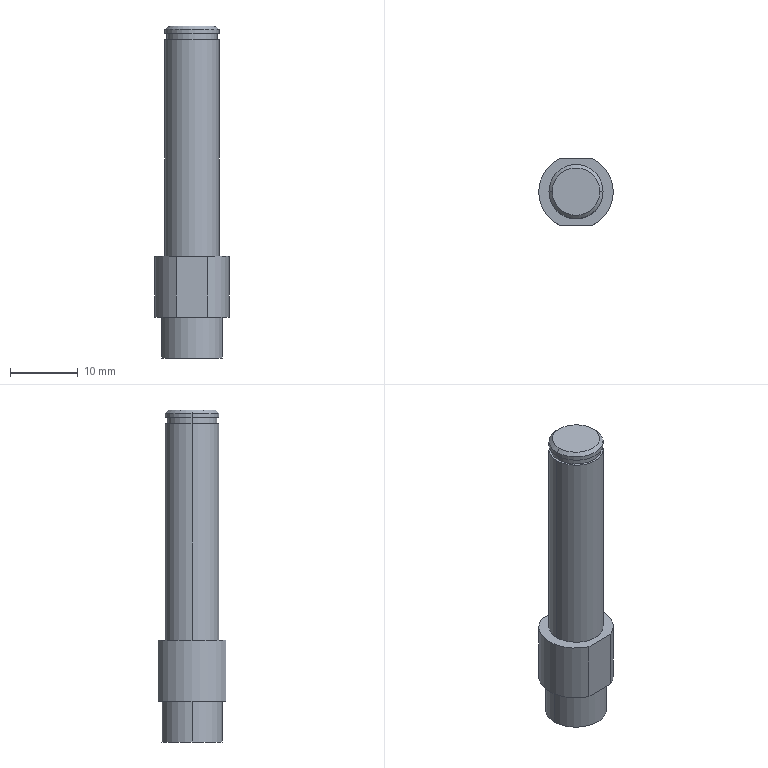Part | STEP file | QA-FC02 | 1 solid | 25 faces | box 11 x 10 x 49 mm | volume 2709 mm3 | cylinder 13 | plane 8 | cone 4 | commonest cylinder face diameters 8 x4 11 x3 4.2 x2 7.4 x2 9 x2
STEP:
#1=CARTESIAN_POINT('',(0.,0.,0.));
#2=DIRECTION('',(0.,0.,1.));
#3=DIRECTION('',(1.,0.,0.));
#4=AXIS2_PLACEMENT_3D('',#1,#2,#3);
#5=CARTESIAN_POINT('',(3.5,0.,34.));
#6=VERTEX_POINT('',#5);
#7=CARTESIAN_POINT('',(-3.5,0.,34.));
#8=VERTEX_POINT('',#7);
#9=CARTESIAN_POINT('',(0.,0.,34.));
#10=DIRECTION('',(0.,0.,1.));
#11=DIRECTION('',(1.,0.,0.));
#12=AXIS2_PLACEMENT_3D('',#9,#10,#11);
#13=CIRCLE('',#12,3.5);
#14=CARTESIAN_POINT('',(0.,0.,34.));
#15=DIRECTION('',(0.,0.,-1.));
#16=DIRECTION('',(-1.,0.,0.));
#17=AXIS2_PLACEMENT_3D('',#14,#15,#16);
#18=CONICAL_SURFACE('',#17,3.5,0.7854);
#19=CARTESIAN_POINT('',(3.142,0.));
#20=DIRECTION('',(-1.,0.));
#21=VECTOR('',#20,1.);
#22=LINE('',#19,#21);
#23=(GEOMETRIC_REPRESENTATION_CONTEXT(2)PARAMETRIC_REPRESENTATION_CONTEXT()REPRESENTATION_CONTEXT('',''));
#24=DEFINITIONAL_REPRESENTATION('',(#22),#23);
#25=PCURVE('',#18,#24);
#26=CARTESIAN_POINT('',(0.,0.,34.));
#27=DIRECTION('',(0.,0.,1.));
#28=DIRECTION('',(1.,0.,0.));
#29=AXIS2_PLACEMENT_3D('',#26,#27,#28);
#30=PLANE('',#29);
#31=CARTESIAN_POINT('',(0.,0.));
#32=DIRECTION('',(1.,0.));
#33=AXIS2_PLACEMENT_2D('',#31,#32);
#34=CIRCLE('',#33,3.5);
#35=(GEOMETRIC_REPRESENTATION_CONTEXT(2)PARAMETRIC_REPRESENTATION_CONTEXT()REPRESENTATION_CONTEXT('',''));
#36=DEFINITIONAL_REPRESENTATION('',(#34),#35);
#37=PCURVE('',#30,#36);
#38=SURFACE_CURVE('',#13,(#25,#37),.PCURVE_S1.);
#39=EDGE_CURVE('',#6,#8,#38,.T.);
#40=ORIENTED_EDGE('',*,*,#39,.F.);
#41=CARTESIAN_POINT('',(4.,0.,33.5));
#42=VERTEX_POINT('',#41);
#43=CARTESIAN_POINT('',(3.5,0.,34.));
#44=DIRECTION('',(0.7071,0.,-0.7071));
#45=VECTOR('',#44,1.);
#46=LINE('',#43,#45);
#47=CARTESIAN_POINT('',(3.142,0.));
#48=DIRECTION('',(0.,1.));
#49=VECTOR('',#48,1.);
#50=LINE('',#47,#49);
#51=(GEOMETRIC_REPRESENTATION_CONTEXT(2)PARAMETRIC_REPRESENTATION_CONTEXT()REPRESENTATION_CONTEXT('',''));
#52=DEFINITIONAL_REPRESENTATION('',(#50),#51);
#53=PCURVE('',#18,#52);
#54=CARTESIAN_POINT('',(0.,0.,34.));
#55=DIRECTION('',(0.,0.,-1.));
#56=DIRECTION('',(-1.,0.,0.));
#57=AXIS2_PLACEMENT_3D('',#54,#55,#56);
#58=CONICAL_SURFACE('',#57,3.5,0.7854);
#59=CARTESIAN_POINT('',(3.142,0.));
#60=DIRECTION('',(0.,1.));
#61=VECTOR('',#60,1.);
#62=LINE('',#59,#61);
#63=(GEOMETRIC_REPRESENTATION_CONTEXT(2)PARAMETRIC_REPRESENTATION_CONTEXT()REPRESENTATION_CONTEXT('',''));
#64=DEFINITIONAL_REPRESENTATION('',(#62),#63);
#65=PCURVE('',#58,#64);
#66=SURFACE_CURVE('',#46,(#53,#65),.PCURVE_S1.);
#67=EDGE_CURVE('',#6,#42,#66,.T.);
#68=ORIENTED_EDGE('',*,*,#67,.T.);
#69=CARTESIAN_POINT('',(-4.,0.,33.5));
#70=VERTEX_POINT('',#69);
#71=CARTESIAN_POINT('',(0.,0.,33.5));
#72=DIRECTION('',(0.,0.,-1.));
#73=DIRECTION('',(1.,0.,0.));
#74=AXIS2_PLACEMENT_3D('',#71,#72,#73);
#75=CIRCLE('',#74,4.);
#76=CARTESIAN_POINT('',(-3.142,0.5));
#77=DIRECTION('',(1.,0.));
#78=VECTOR('',#77,1.);
#79=LINE('',#76,#78);
#80=(GEOMETRIC_REPRESENTATION_CONTEXT(2)PARAMETRIC_REPRESENTATION_CONTEXT()REPRESENTATION_CONTEXT('',''));
#81=DEFINITIONAL_REPRESENTATION('',(#79),#80);
#82=PCURVE('',#18,#81);
#83=CARTESIAN_POINT('',(0.,0.,34.));
#84=DIRECTION('',(0.,0.,-1.));
#85=DIRECTION('',(-1.,0.,0.));
#86=AXIS2_PLACEMENT_3D('',#83,#84,#85);
#87=CYLINDRICAL_SURFACE('',#86,4.);
#88=CARTESIAN_POINT('',(-3.142,0.5));
#89=DIRECTION('',(1.,0.));
#90=VECTOR('',#89,1.);
#91=LINE('',#88,#90);
#92=(GEOMETRIC_REPRESENTATION_CONTEXT(2)PARAMETRIC_REPRESENTATION_CONTEXT()REPRESENTATION_CONTEXT('',''));
#93=DEFINITIONAL_REPRESENTATION('',(#91),#92);
#94=PCURVE('',#87,#93);
#95=SURFACE_CURVE('',#75,(#82,#94),.PCURVE_S1.);
#96=EDGE_CURVE('',#70,#42,#95,.T.);
#97=ORIENTED_EDGE('',*,*,#96,.F.);
#98=CARTESIAN_POINT('',(-3.5,0.,34.));
#99=DIRECTION('',(-0.7071,0.,-0.7071));
#100=VECTOR('',#99,1.);
#101=LINE('',#98,#100);
#102=CARTESIAN_POINT('',(0.,0.));
#103=DIRECTION('',(0.,1.));
#104=VECTOR('',#103,1.);
#105=LINE('',#102,#104);
#106=(GEOMETRIC_REPRESENTATION_CONTEXT(2)PARAMETRIC_REPRESENTATION_CONTEXT()REPRESENTATION_CONTEXT('',''));
#107=DEFINITIONAL_REPRESENTATION('',(#105),#106);
#108=PCURVE('',#18,#107);
#109=CARTESIAN_POINT('',(6.283,0.));
#110=DIRECTION('',(0.,1.));
#111=VECTOR('',#110,1.);
#112=LINE('',#109,#111);
#113=(GEOMETRIC_REPRESENTATION_CONTEXT(2)PARAMETRIC_REPRESENTATION_CONTEXT()REPRESENTATION_CONTEXT('',''));
#114=DEFINITIONAL_REPRESENTATION('',(#112),#113);
#115=PCURVE('',#58,#114);
#116=SURFACE_CURVE('',#101,(#108,#115),.PCURVE_S1.);
#117=EDGE_CURVE('',#8,#70,#116,.T.);
#118=ORIENTED_EDGE('',*,*,#117,.F.);
#119=EDGE_LOOP('',(#40,#68,#97,#118));
#120=FACE_BOUND('',#119,.T.);
#121=ADVANCED_FACE('',(#120),#18,.T.);
#122=ORIENTED_EDGE('',*,*,#96,.T.);
#123=CARTESIAN_POINT('',(4.,0.,32.9));
#124=VERTEX_POINT('',#123);
#125=CARTESIAN_POINT('',(4.,0.,34.));
#126=DIRECTION('',(0.,0.,-1.));
#127=VECTOR('',#126,1.);
#128=LINE('',#125,#127);
#129=CARTESIAN_POINT('',(3.142,0.));
#130=DIRECTION('',(0.,1.));
#131=VECTOR('',#130,1.);
#132=LINE('',#129,#131);
#133=(GEOMETRIC_REPRESENTATION_CONTEXT(2)PARAMETRIC_REPRESENTATION_CONTEXT()REPRESENTATION_CONTEXT('',''));
#134=DEFINITIONAL_REPRESENTATION('',(#132),#133);
#135=PCURVE('',#87,#134);
#136=CARTESIAN_POINT('',(0.,0.,34.));
#137=DIRECTION('',(0.,0.,-1.));
#138=DIRECTION('',(-1.,0.,0.));
#139=AXIS2_PLACEMENT_3D('',#136,#137,#138);
#140=CYLINDRICAL_SURFACE('',#139,4.);
#141=CARTESIAN_POINT('',(3.142,0.));
#142=DIRECTION('',(0.,1.));
#143=VECTOR('',#142,1.);
#144=LINE('',#141,#143);
#145=(GEOMETRIC_REPRESENTATION_CONTEXT(2)PARAMETRIC_REPRESENTATION_CONTEXT()REPRESENTATION_CONTEXT('',''));
#146=DEFINITIONAL_REPRESENTATION('',(#144),#145);
#147=PCURVE('',#140,#146);
#148=SURFACE_CURVE('',#128,(#135,#147),.PCURVE_S1.);
#149=EDGE_CURVE('',#42,#124,#148,.T.);
#150=ORIENTED_EDGE('',*,*,#149,.T.);
#151=CARTESIAN_POINT('',(-4.,0.,32.9));
#152=VERTEX_POINT('',#151);
#153=CARTESIAN_POINT('',(0.,0.,32.9));
#154=DIRECTION('',(0.,0.,1.));
#155=DIRECTION('',(1.,0.,0.));
#156=AXIS2_PLACEMENT_3D('',#153,#154,#155);
#157=CIRCLE('',#156,4.);
#158=CARTESIAN_POINT('',(3.142,1.1));
#159=DIRECTION('',(-1.,0.));
#160=VECTOR('',#159,1.);
#161=LINE('',#158,#160);
#162=(GEOMETRIC_REPRESENTATION_CONTEXT(2)PARAMETRIC_REPRESENTATION_CONTEXT()REPRESENTATION_CONTEXT('',''));
#163=DEFINITIONAL_REPRESENTATION('',(#161),#162);
#164=PCURVE('',#87,#163);
#165=CARTESIAN_POINT('',(0.,0.,32.9));
#166=DIRECTION('',(0.,0.,1.));
#167=DIRECTION('',(1.,0.,0.));
#168=AXIS2_PLACEMENT_3D('',#165,#166,#167);
#169=PLANE('',#168);
#170=CARTESIAN_POINT('',(0.,0.));
#171=DIRECTION('',(1.,0.));
#172=AXIS2_PLACEMENT_2D('',#170,#171);
#173=CIRCLE('',#172,4.);
#174=(GEOMETRIC_REPRESENTATION_CONTEXT(2)PARAMETRIC_REPRESENTATION_CONTEXT()REPRESENTATION_CONTEXT('',''));
#175=DEFINITIONAL_REPRESENTATION('',(#173),#174);
#176=PCURVE('',#169,#175);
#177=SURFACE_CURVE('',#157,(#164,#176),.PCURVE_S1.);
#178=EDGE_CURVE('',#124,#152,#177,.T.);
#179=ORIENTED_EDGE('',*,*,#178,.T.);
#180=CARTESIAN_POINT('',(-4.,0.,34.));
#181=DIRECTION('',(0.,0.,-1.));
#182=VECTOR('',#181,1.);
#183=LINE('',#180,#182);
#184=CARTESIAN_POINT('',(0.,0.));
#185=DIRECTION('',(0.,1.));
#186=VECTOR('',#185,1.);
#187=LINE('',#184,#186);
#188=(GEOMETRIC_REPRESENTATION_CONTEXT(2)PARAMETRIC_REPRESENTATION_CONTEXT()REPRESENTATION_CONTEXT('',''));
#189=DEFINITIONAL_REPRESENTATION('',(#187),#188);
#190=PCURVE('',#87,#189);
#191=CARTESIAN_POINT('',(6.283,0.));
#192=DIRECTION('',(0.,1.));
#193=VECTOR('',#192,1.);
#194=LINE('',#191,#193);
#195=(GEOMETRIC_REPRESENTATION_CONTEXT(2)PARAMETRIC_REPRESENTATION_CONTEXT()REPRESENTATION_CONTEXT('',''));
#196=DEFINITIONAL_REPRESENTATION('',(#194),#195);
#197=PCURVE('',#140,#196);
#198=SURFACE_CURVE('',#183,(#190,#197),.PCURVE_S1.);
#199=EDGE_CURVE('',#70,#152,#198,.T.);
#200=ORIENTED_EDGE('',*,*,#199,.F.);
#201=EDGE_LOOP('',(#122,#150,#179,#200));
#202=FACE_BOUND('',#201,.T.);
#203=ADVANCED_FACE('',(#202),#87,.T.);
#204=CARTESIAN_POINT('',(3.7,0.,32.9));
#205=VERTEX_POINT('',#204);
#206=CARTESIAN_POINT('',(-3.7,0.,32.9));
#207=VERTEX_POINT('',#206);
#208=CARTESIAN_POINT('',(0.,0.,32.9));
#209=DIRECTION('',(0.,0.,1.));
#210=DIRECTION('',(1.,0.,0.));
#211=AXIS2_PLACEMENT_3D('',#208,#209,#210);
#212=CIRCLE('',#211,3.7);
#213=CARTESIAN_POINT('',(0.,0.,32.9));
#214=DIRECTION('',(0.,0.,-1.));
#215=DIRECTION('',(-1.,0.,0.));
#216=AXIS2_PLACEMENT_3D('',#213,#214,#215);
#217=CYLINDRICAL_SURFACE('',#216,3.7);
#218=CARTESIAN_POINT('',(3.142,0.));
#219=DIRECTION('',(-1.,0.));
#220=VECTOR('',#219,1.);
#221=LINE('',#218,#220);
#222=(GEOMETRIC_REPRESENTATION_CONTEXT(2)PARAMETRIC_REPRESENTATION_CONTEXT()REPRESENTATION_CONTEXT('',''));
#223=DEFINITIONAL_REPRESENTATION('',(#221),#222);
#224=PCURVE('',#217,#223);
#225=CARTESIAN_POINT('',(0.,0.));
#226=DIRECTION('',(1.,0.));
#227=AXIS2_PLACEMENT_2D('',#225,#226);
#228=CIRCLE('',#227,3.7);
#229=(GEOMETRIC_REPRESENTATION_CONTEXT(2)PARAMETRIC_REPRESENTATION_CONTEXT()REPRESENTATION_CONTEXT('',''));
#230=DEFINITIONAL_REPRESENTATION('',(#228),#229);
#231=PCURVE('',#169,#230);
#232=SURFACE_CURVE('',#212,(#224,#231),.PCURVE_S1.);
#233=EDGE_CURVE('',#205,#207,#232,.T.);
#234=ORIENTED_EDGE('',*,*,#233,.F.);
#235=CARTESIAN_POINT('',(3.7,0.,32.));
#236=VERTEX_POINT('',#235);
#237=CARTESIAN_POINT('',(3.7,0.,32.9));
#238=DIRECTION('',(0.,0.,-1.));
#239=VECTOR('',#238,1.);
#240=LINE('',#237,#239);
#241=CARTESIAN_POINT('',(3.142,0.));
#242=DIRECTION('',(0.,1.));
#243=VECTOR('',#242,1.);
#244=LINE('',#241,#243);
#245=(GEOMETRIC_REPRESENTATION_CONTEXT(2)PARAMETRIC_REPRESENTATION_CONTEXT()REPRESENTATION_CONTEXT('',''));
#246=DEFINITIONAL_REPRESENTATION('',(#244),#245);
#247=PCURVE('',#217,#246);
#248=CARTESIAN_POINT('',(0.,0.,32.9));
#249=DIRECTION('',(0.,0.,-1.));
#250=DIRECTION('',(-1.,0.,0.));
#251=AXIS2_PLACEMENT_3D('',#248,#249,#250);
#252=CYLINDRICAL_SURFACE('',#251,3.7);
#253=CARTESIAN_POINT('',(3.142,0.));
#254=DIRECTION('',(0.,1.));
#255=VECTOR('',#254,1.);
#256=LINE('',#253,#255);
#257=(GEOMETRIC_REPRESENTATION_CONTEXT(2)PARAMETRIC_REPRESENTATION_CONTEXT()REPRESENTATION_CONTEXT('',''));
#258=DEFINITIONAL_REPRESENTATION('',(#256),#257);
#259=PCURVE('',#252,#258);
#260=SURFACE_CURVE('',#240,(#247,#259),.PCURVE_S1.);
#261=EDGE_CURVE('',#205,#236,#260,.T.);
#262=ORIENTED_EDGE('',*,*,#261,.T.);
#263=CARTESIAN_POINT('',(-3.7,0.,32.));
#264=VERTEX_POINT('',#263);
#265=CARTESIAN_POINT('',(0.,0.,32.));
#266=DIRECTION('',(0.,0.,1.));
#267=DIRECTION('',(1.,0.,0.));
#268=AXIS2_PLACEMENT_3D('',#265,#266,#267);
#269=CIRCLE('',#268,3.7);
#270=CARTESIAN_POINT('',(3.142,0.9));
#271=DIRECTION('',(-1.,0.));
#272=VECTOR('',#271,1.);
#273=LINE('',#270,#272);
#274=(GEOMETRIC_REPRESENTATION_CONTEXT(2)PARAMETRIC_REPRESENTATION_CONTEXT()REPRESENTATION_CONTEXT('',''));
#275=DEFINITIONAL_REPRESENTATION('',(#273),#274);
#276=PCURVE('',#217,#275);
#277=CARTESIAN_POINT('',(0.,0.,32.));
#278=DIRECTION('',(0.,0.,1.));
#279=DIRECTION('',(1.,0.,0.));
#280=AXIS2_PLACEMENT_3D('',#277,#278,#279);
#281=PLANE('',#280);
#282=CARTESIAN_POINT('',(0.,0.));
#283=DIRECTION('',(1.,0.));
#284=AXIS2_PLACEMENT_2D('',#282,#283);
#285=CIRCLE('',#284,3.7);
#286=(GEOMETRIC_REPRESENTATION_CONTEXT(2)PARAMETRIC_REPRESENTATION_CONTEXT()REPRESENTATION_CONTEXT('',''));
#287=DEFINITIONAL_REPRESENTATION('',(#285),#286);
#288=PCURVE('',#281,#287);
#289=SURFACE_CURVE('',#269,(#276,#288),.PCURVE_S1.);
#290=EDGE_CURVE('',#236,#264,#289,.T.);
#291=ORIENTED_EDGE('',*,*,#290,.T.);
#292=CARTESIAN_POINT('',(-3.7,0.,32.9));
#293=DIRECTION('',(0.,0.,-1.));
#294=VECTOR('',#293,1.);
#295=LINE('',#292,#294);
#296=CARTESIAN_POINT('',(0.,0.));
#297=DIRECTION('',(0.,1.));
#298=VECTOR('',#297,1.);
#299=LINE('',#296,#298);
#300=(GEOMETRIC_REPRESENTATION_CONTEXT(2)PARAMETRIC_REPRESENTATION_CONTEXT()REPRESENTATION_CONTEXT('',''));
#301=DEFINITIONAL_REPRESENTATION('',(#299),#300);
#302=PCURVE('',#217,#301);
#303=CARTESIAN_POINT('',(6.283,0.));
#304=DIRECTION('',(0.,1.));
#305=VECTOR('',#304,1.);
#306=LINE('',#303,#305);
#307=(GEOMETRIC_REPRESENTATION_CONTEXT(2)PARAMETRIC_REPRESENTATION_CONTEXT()REPRESENTATION_CONTEXT('',''));
#308=DEFINITIONAL_REPRESENTATION('',(#306),#307);
#309=PCURVE('',#252,#308);
#310=SURFACE_CURVE('',#295,(#302,#309),.PCURVE_S1.);
#311=EDGE_CURVE('',#207,#264,#310,.T.);
#312=ORIENTED_EDGE('',*,*,#311,.F.);
#313=EDGE_LOOP('',(#234,#262,#291,#312));
#314=FACE_BOUND('',#313,.T.);
#315=ADVANCED_FACE('',(#314),#217,.T.);
#316=CARTESIAN_POINT('',(-2.1,0.,-1.));
#317=VERTEX_POINT('',#316);
#318=CARTESIAN_POINT('',(-2.1,0.,-15.));
#319=VERTEX_POINT('',#318);
#320=CARTESIAN_POINT('',(-2.1,0.,-15.));
#321=DIRECTION('',(0.,0.,-1.));
#322=VECTOR('',#321,1.);
#323=LINE('',#320,#322);
#324=CARTESIAN_POINT('',(0.,0.,-15.));
#325=DIRECTION('',(0.,0.,-1.));
#326=DIRECTION('',(-1.,0.,0.));
#327=AXIS2_PLACEMENT_3D('',#324,#325,#326);
#328=CYLINDRICAL_SURFACE('',#327,2.1);
#329=CARTESIAN_POINT('',(6.283,0.));
#330=DIRECTION('',(0.,1.));
#331=VECTOR('',#330,1.);
#332=LINE('',#329,#331);
#333=(GEOMETRIC_REPRESENTATION_CONTEXT(2)PARAMETRIC_REPRESENTATION_CONTEXT()REPRESENTATION_CONTEXT('',''));
#334=DEFINITIONAL_REPRESENTATION('',(#332),#333);
#335=PCURVE('',#328,#334);
#336=CARTESIAN_POINT('',(0.,0.,-15.));
#337=DIRECTION('',(0.,0.,-1.));
#338=DIRECTION('',(-1.,0.,0.));
#339=AXIS2_PLACEMENT_3D('',#336,#337,#338);
#340=CYLINDRICAL_SURFACE('',#339,2.1);
#341=CARTESIAN_POINT('',(0.,0.));
#342=DIRECTION('',(0.,1.));
#343=VECTOR('',#342,1.);
#344=LINE('',#341,#343);
#345=(GEOMETRIC_REPRESENTATION_CONTEXT(2)PARAMETRIC_REPRESENTATION_CONTEXT()REPRESENTATION_CONTEXT('',''));
#346=DEFINITIONAL_REPRESENTATION('',(#344),#345);
#347=PCURVE('',#340,#346);
#348=SURFACE_CURVE('',#323,(#335,#347),.PCURVE_S1.);
#349=EDGE_CURVE('',#317,#319,#348,.T.);
#350=ORIENTED_EDGE('',*,*,#349,.T.);
#351=CARTESIAN_POINT('',(2.1,0.,-15.));
#352=VERTEX_POINT('',#351);
#353=CARTESIAN_POINT('',(0.,0.,-15.));
#354=DIRECTION('',(0.,0.,-1.));
#355=DIRECTION('',(-1.,0.,0.));
#356=AXIS2_PLACEMENT_3D('',#353,#354,#355);
#357=CIRCLE('',#356,2.1);
#358=CARTESIAN_POINT('',(0.,0.));
#359=DIRECTION('',(1.,0.));
#360=VECTOR('',#359,1.);
#361=LINE('',#358,#360);
#362=(GEOMETRIC_REPRESENTATION_CONTEXT(2)PARAMETRIC_REPRESENTATION_CONTEXT()REPRESENTATION_CONTEXT('',''));
#363=DEFINITIONAL_REPRESENTATION('',(#361),#362);
#364=PCURVE('',#328,#363);
#365=CARTESIAN_POINT('',(0.,0.,-15.));
#366=DIRECTION('',(0.,0.,-1.));
#367=DIRECTION('',(-1.,0.,0.));
#368=AXIS2_PLACEMENT_3D('',#365,#366,#367);
#369=PLANE('',#368);
#370=CARTESIAN_POINT('',(0.,0.));
#371=DIRECTION('',(1.,0.));
#372=AXIS2_PLACEMENT_2D('',#370,#371);
#373=CIRCLE('',#372,2.1);
#374=(GEOMETRIC_REPRESENTATION_CONTEXT(2)PARAMETRIC_REPRESENTATION_CONTEXT()REPRESENTATION_CONTEXT('',''));
#375=DEFINITIONAL_REPRESENTATION('',(#373),#374);
#376=PCURVE('',#369,#375);
#377=SURFACE_CURVE('',#357,(#364,#376),.PCURVE_S1.);
#378=EDGE_CURVE('',#352,#319,#377,.T.);
#379=ORIENTED_EDGE('',*,*,#378,.F.);
#380=CARTESIAN_POINT('',(2.1,0.,-1.));
#381=VERTEX_POINT('',#380);
#382=CARTESIAN_POINT('',(2.1,0.,-15.));
#383=DIRECTION('',(0.,0.,-1.));
#384=VECTOR('',#383,1.);
#385=LINE('',#382,#384);
#386=CARTESIAN_POINT('',(3.142,0.));
#387=DIRECTION('',(0.,1.));
#388=VECTOR('',#387,1.);
#389=LINE('',#386,#388);
#390=(GEOMETRIC_REPRESENTATION_CONTEXT(2)PARAMETRIC_REPRESENTATION_CONTEXT()REPRESENTATION_CONTEXT('',''));
#391=DEFINITIONAL_REPRESENTATION('',(#389),#390);
#392=PCURVE('',#328,#391);
#393=CARTESIAN_POINT('',(3.142,0.));
#394=DIRECTION('',(0.,1.));
#395=VECTOR('',#394,1.);
#396=LINE('',#393,#395);
#397=(GEOMETRIC_REPRESENTATION_CONTEXT(2)PARAMETRIC_REPRESENTATION_CONTEXT()REPRESENTATION_CONTEXT('',''));
#398=DEFINITIONAL_REPRESENTATION('',(#396),#397);
#399=PCURVE('',#340,#398);
#400=SURFACE_CURVE('',#385,(#392,#399),.PCURVE_S1.);
#401=EDGE_CURVE('',#381,#352,#400,.T.);
#402=ORIENTED_EDGE('',*,*,#401,.F.);
#403=CARTESIAN_POINT('',(0.,0.,-1.));
#404=DIRECTION('',(0.,0.,-1.));
#405=DIRECTION('',(-1.,0.,0.));
#406=AXIS2_PLACEMENT_3D('',#403,#404,#405);
#407=CIRCLE('',#406,2.1);
#408=CARTESIAN_POINT('',(0.,-14.));
#409=DIRECTION('',(1.,0.));
#410=VECTOR('',#409,1.);
#411=LINE('',#408,#410);
#412=(GEOMETRIC_REPRESENTATION_CONTEXT(2)PARAMETRIC_REPRESENTATION_CONTEXT()REPRESENTATION_CONTEXT('',''));
#413=DEFINITIONAL_REPRESENTATION('',(#411),#412);
#414=PCURVE('',#328,#413);
#415=CARTESIAN_POINT('',(0.,0.,-1.));
#416=DIRECTION('',(0.,0.,-1.));
#417=DIRECTION('',(-1.,0.,0.));
#418=AXIS2_PLACEMENT_3D('',#415,#416,#417);
#419=CONICAL_SURFACE('',#418,2.1,1.03);
#420=CARTESIAN_POINT('',(0.,0.));
#421=DIRECTION('',(1.,0.));
#422=VECTOR('',#421,1.);
#423=LINE('',#420,#422);
#424=(GEOMETRIC_REPRESENTATION_CONTEXT(2)PARAMETRIC_REPRESENTATION_CONTEXT()REPRESENTATION_CONTEXT('',''));
#425=DEFINITIONAL_REPRESENTATION('',(#423),#424);
#426=PCURVE('',#419,#425);
#427=SURFACE_CURVE('',#407,(#414,#426),.PCURVE_S1.);
#428=EDGE_CURVE('',#381,#317,#427,.T.);
#429=ORIENTED_EDGE('',*,*,#428,.T.);
#430=EDGE_LOOP('',(#350,#379,#402,#429));
#431=FACE_BOUND('',#430,.F.);
#432=ADVANCED_FACE('',(#431),#328,.F.);
#433=ORIENTED_EDGE('',*,*,#428,.F.);
#434=CARTESIAN_POINT('',(0.,0.,0.2618));
#435=VERTEX_POINT('',#434);
#436=CARTESIAN_POINT('',(2.1,0.,-1.));
#437=DIRECTION('',(0.8572,0.,-0.515));
#438=VECTOR('',#437,1.);
#439=LINE('',#436,#438);
#440=CARTESIAN_POINT('',(3.142,0.));
#441=DIRECTION('',(0.,1.));
#442=VECTOR('',#441,1.);
#443=LINE('',#440,#442);
#444=(GEOMETRIC_REPRESENTATION_CONTEXT(2)PARAMETRIC_REPRESENTATION_CONTEXT()REPRESENTATION_CONTEXT('',''));
#445=DEFINITIONAL_REPRESENTATION('',(#443),#444);
#446=PCURVE('',#419,#445);
#447=CARTESIAN_POINT('',(0.,0.,-1.));
#448=DIRECTION('',(0.,0.,-1.));
#449=DIRECTION('',(-1.,0.,0.));
#450=AXIS2_PLACEMENT_3D('',#447,#448,#449);
#451=CONICAL_SURFACE('',#450,2.1,1.03);
#452=CARTESIAN_POINT('',(3.142,0.));
#453=DIRECTION('',(0.,1.));
#454=VECTOR('',#453,1.);
#455=LINE('',#452,#454);
#456=(GEOMETRIC_REPRESENTATION_CONTEXT(2)PARAMETRIC_REPRESENTATION_CONTEXT()REPRESENTATION_CONTEXT('',''));
#457=DEFINITIONAL_REPRESENTATION('',(#455),#456);
#458=PCURVE('',#451,#457);
#459=SURFACE_CURVE('',#439,(#446,#458),.PCURVE_S1.);
#460=EDGE_CURVE('',#435,#381,#459,.T.);
#461=ORIENTED_EDGE('',*,*,#460,.F.);
#462=CARTESIAN_POINT('',(-2.1,0.,-1.));
#463=DIRECTION('',(-0.8572,0.,-0.515));
#464=VECTOR('',#463,1.);
#465=LINE('',#462,#464);
#466=CARTESIAN_POINT('',(6.283,0.));
#467=DIRECTION('',(0.,1.));
#468=VECTOR('',#467,1.);
#469=LINE('',#466,#468);
#470=(GEOMETRIC_REPRESENTATION_CONTEXT(2)PARAMETRIC_REPRESENTATION_CONTEXT()REPRESENTATION_CONTEXT('',''));
#471=DEFINITIONAL_REPRESENTATION('',(#469),#470);
#472=PCURVE('',#419,#471);
#473=CARTESIAN_POINT('',(0.,0.));
#474=DIRECTION('',(0.,1.));
#475=VECTOR('',#474,1.);
#476=LINE('',#473,#475);
#477=(GEOMETRIC_REPRESENTATION_CONTEXT(2)PARAMETRIC_REPRESENTATION_CONTEXT()REPRESENTATION_CONTEXT('',''));
#478=DEFINITIONAL_REPRESENTATION('',(#476),#477);
#479=PCURVE('',#451,#478);
#480=SURFACE_CURVE('',#465,(#472,#479),.PCURVE_S1.);
#481=EDGE_CURVE('',#435,#317,#480,.T.);
#482=ORIENTED_EDGE('',*,*,#481,.T.);
#483=EDGE_LOOP('',(#433,#461,#482));
#484=FACE_BOUND('',#483,.F.);
#485=ADVANCED_FACE('',(#484),#419,.F.);
#486=CARTESIAN_POINT('',(-4.5,0.,-15.));
#487=VERTEX_POINT('',#486);
#488=CARTESIAN_POINT('',(4.5,0.,-15.));
#489=VERTEX_POINT('',#488);
#490=CARTESIAN_POINT('',(0.,0.,-15.));
#491=DIRECTION('',(0.,0.,-1.));
#492=DIRECTION('',(-1.,0.,0.));
#493=AXIS2_PLACEMENT_3D('',#490,#491,#492);
#494=CIRCLE('',#493,4.5);
#495=CARTESIAN_POINT('',(0.,0.,-15.));
#496=DIRECTION('',(0.,0.,1.));
#497=DIRECTION('',(1.,0.,0.));
#498=AXIS2_PLACEMENT_3D('',#495,#496,#497);
#499=CYLINDRICAL_SURFACE('',#498,4.5);
#500=CARTESIAN_POINT('',(3.142,0.));
#501=DIRECTION('',(-1.,0.));
#502=VECTOR('',#501,1.);
#503=LINE('',#500,#502);
#504=(GEOMETRIC_REPRESENTATION_CONTEXT(2)PARAMETRIC_REPRESENTATION_CONTEXT()REPRESENTATION_CONTEXT('',''));
#505=DEFINITIONAL_REPRESENTATION('',(#503),#504);
#506=PCURVE('',#499,#505);
#507=CARTESIAN_POINT('',(0.,0.));
#508=DIRECTION('',(1.,0.));
#509=AXIS2_PLACEMENT_2D('',#507,#508);
#510=CIRCLE('',#509,4.5);
#511=(GEOMETRIC_REPRESENTATION_CONTEXT(2)PARAMETRIC_REPRESENTATION_CONTEXT()REPRESENTATION_CONTEXT('',''));
#512=DEFINITIONAL_REPRESENTATION('',(#510),#511);
#513=PCURVE('',#369,#512);
#514=SURFACE_CURVE('',#494,(#506,#513),.PCURVE_S1.);
#515=EDGE_CURVE('',#487,#489,#514,.T.);
#516=ORIENTED_EDGE('',*,*,#515,.F.);
#517=CARTESIAN_POINT('',(-4.5,0.,-9.));
#518=VERTEX_POINT('',#517);
#519=CARTESIAN_POINT('',(-4.5,0.,-15.));
#520=DIRECTION('',(0.,0.,1.));
#521=VECTOR('',#520,1.);
#522=LINE('',#519,#521);
#523=CARTESIAN_POINT('',(3.142,0.));
#524=DIRECTION('',(0.,1.));
#525=VECTOR('',#524,1.);
#526=LINE('',#523,#525);
#527=(GEOMETRIC_REPRESENTATION_CONTEXT(2)PARAMETRIC_REPRESENTATION_CONTEXT()REPRESENTATION_CONTEXT('',''));
#528=DEFINITIONAL_REPRESENTATION('',(#526),#527);
#529=PCURVE('',#499,#528);
#530=CARTESIAN_POINT('',(0.,0.,-15.));
#531=DIRECTION('',(0.,0.,1.));
#532=DIRECTION('',(1.,0.,0.));
#533=AXIS2_PLACEMENT_3D('',#530,#531,#532);
#534=CYLINDRICAL_SURFACE('',#533,4.5);
#535=CARTESIAN_POINT('',(3.142,0.));
#536=DIRECTION('',(0.,1.));
#537=VECTOR('',#536,1.);
#538=LINE('',#535,#537);
#539=(GEOMETRIC_REPRESENTATION_CONTEXT(2)PARAMETRIC_REPRESENTATION_CONTEXT()REPRESENTATION_CONTEXT('',''));
#540=DEFINITIONAL_REPRESENTATION('',(#538),#539);
#541=PCURVE('',#534,#540);
#542=SURFACE_CURVE('',#522,(#529,#541),.PCURVE_S1.);
#543=EDGE_CURVE('',#487,#518,#542,.T.);
#544=ORIENTED_EDGE('',*,*,#543,.T.);
#545=CARTESIAN_POINT('',(4.5,0.,-9.));
#546=VERTEX_POINT('',#545);
#547=CARTESIAN_POINT('',(0.,0.,-9.));
#548=DIRECTION('',(0.,0.,-1.));
#549=DIRECTION('',(-1.,0.,0.));
#550=AXIS2_PLACEMENT_3D('',#547,#548,#549);
#551=CIRCLE('',#550,4.5);
#552=CARTESIAN_POINT('',(3.142,6.));
#553=DIRECTION('',(-1.,0.));
#554=VECTOR('',#553,1.);
#555=LINE('',#552,#554);
#556=(GEOMETRIC_REPRESENTATION_CONTEXT(2)PARAMETRIC_REPRESENTATION_CONTEXT()REPRESENTATION_CONTEXT('',''));
#557=DEFINITIONAL_REPRESENTATION('',(#555),#556);
#558=PCURVE('',#499,#557);
#559=CARTESIAN_POINT('',(0.,0.,-9.));
#560=DIRECTION('',(0.,0.,-1.));
#561=DIRECTION('',(-1.,0.,0.));
#562=AXIS2_PLACEMENT_3D('',#559,#560,#561);
#563=PLANE('',#562);
#564=CARTESIAN_POINT('',(0.,0.));
#565=DIRECTION('',(1.,0.));
#566=AXIS2_PLACEMENT_2D('',#564,#565);
#567=CIRCLE('',#566,4.5);
#568=(GEOMETRIC_REPRESENTATION_CONTEXT(2)PARAMETRIC_REPRESENTATION_CONTEXT()REPRESENTATION_CONTEXT('',''));
#569=DEFINITIONAL_REPRESENTATION('',(#567),#568);
#570=PCURVE('',#563,#569);
#571=SURFACE_CURVE('',#551,(#558,#570),.PCURVE_S1.);
#572=EDGE_CURVE('',#518,#546,#571,.T.);
#573=ORIENTED_EDGE('',*,*,#572,.T.);
#574=CARTESIAN_POINT('',(4.5,0.,-15.));
#575=DIRECTION('',(0.,0.,1.));
#576=VECTOR('',#575,1.);
#577=LINE('',#574,#576);
#578=CARTESIAN_POINT('',(0.,0.));
#579=DIRECTION('',(0.,1.));
#580=VECTOR('',#579,1.);
#581=LINE('',#578,#580);
#582=(GEOMETRIC_REPRESENTATION_CONTEXT(2)PARAMETRIC_REPRESENTATION_CONTEXT()REPRESENTATION_CONTEXT('',''));
#583=DEFINITIONAL_REPRESENTATION('',(#581),#582);
#584=PCURVE('',#499,#583);
#585=CARTESIAN_POINT('',(6.283,0.));
#586=DIRECTION('',(0.,1.));
#587=VECTOR('',#586,1.);
#588=LINE('',#585,#587);
#589=(GEOMETRIC_REPRESENTATION_CONTEXT(2)PARAMETRIC_REPRESENTATION_CONTEXT()REPRESENTATION_CONTEXT('',''));
#590=DEFINITIONAL_REPRESENTATION('',(#588),#589);
#591=PCURVE('',#534,#590);
#592=SURFACE_CURVE('',#577,(#584,#591),.PCURVE_S1.);
#593=EDGE_CURVE('',#489,#546,#592,.T.);
#594=ORIENTED_EDGE('',*,*,#593,.F.);
#595=EDGE_LOOP('',(#516,#544,#573,#594));
#596=FACE_BOUND('',#595,.T.);
#597=ADVANCED_FACE('',(#596),#499,.T.);
#598=CARTESIAN_POINT('',(5.5,0.,-9.));
#599=VERTEX_POINT('',#598);
#600=CARTESIAN_POINT('',(2.291,-5.,-9.));
#601=VERTEX_POINT('',#600);
#602=CARTESIAN_POINT('',(0.,0.,-9.));
#603=DIRECTION('',(0.,0.,-1.));
#604=DIRECTION('',(-1.,0.,0.));
#605=AXIS2_PLACEMENT_3D('',#602,#603,#604);
#606=CIRCLE('',#605,5.5);
#607=CARTESIAN_POINT('',(0.,0.,-9.));
#608=DIRECTION('',(0.,0.,1.));
#609=DIRECTION('',(1.,0.,0.));
#610=AXIS2_PLACEMENT_3D('',#607,#608,#609);
#611=CYLINDRICAL_SURFACE('',#610,5.5);
#612=CARTESIAN_POINT('',(9.425,0.));
#613=DIRECTION('',(-1.,0.));
#614=VECTOR('',#613,1.);
#615=LINE('',#612,#614);
#616=(GEOMETRIC_REPRESENTATION_CONTEXT(2)PARAMETRIC_REPRESENTATION_CONTEXT()REPRESENTATION_CONTEXT('',''));
#617=DEFINITIONAL_REPRESENTATION('',(#615),#616);
#618=PCURVE('',#611,#617);
#619=CARTESIAN_POINT('',(0.,0.));
#620=DIRECTION('',(1.,0.));
#621=AXIS2_PLACEMENT_2D('',#619,#620);
#622=CIRCLE('',#621,5.5);
#623=(GEOMETRIC_REPRESENTATION_CONTEXT(2)PARAMETRIC_REPRESENTATION_CONTEXT()REPRESENTATION_CONTEXT('',''));
#624=DEFINITIONAL_REPRESENTATION('',(#622),#623);
#625=PCURVE('',#563,#624);
#626=SURFACE_CURVE('',#606,(#618,#625),.PCURVE_S1.);
#627=EDGE_CURVE('',#599,#601,#626,.T.);
#628=ORIENTED_EDGE('',*,*,#627,.F.);
#629=CARTESIAN_POINT('',(5.5,0.,0.));
#630=VERTEX_POINT('',#629);
#631=CARTESIAN_POINT('',(5.5,0.,-9.));
#632=DIRECTION('',(0.,0.,1.));
#633=VECTOR('',#632,1.);
#634=LINE('',#631,#633);
#635=CARTESIAN_POINT('',(6.283,0.));
#636=DIRECTION('',(0.,1.));
#637=VECTOR('',#636,1.);
#638=LINE('',#635,#637);
#639=(GEOMETRIC_REPRESENTATION_CONTEXT(2)PARAMETRIC_REPRESENTATION_CONTEXT()REPRESENTATION_CONTEXT('',''));
#640=DEFINITIONAL_REPRESENTATION('',(#638),#639);
#641=PCURVE('',#611,#640);
#642=CARTESIAN_POINT('',(0.,0.,-9.));
#643=DIRECTION('',(0.,0.,1.));
#644=DIRECTION('',(1.,0.,0.));
#645=AXIS2_PLACEMENT_3D('',#642,#643,#644);
#646=CYLINDRICAL_SURFACE('',#645,5.5);
#647=CARTESIAN_POINT('',(0.,0.));
#648=DIRECTION('',(0.,1.));
#649=VECTOR('',#648,1.);
#650=LINE('',#647,#649);
#651=(GEOMETRIC_REPRESENTATION_CONTEXT(2)PARAMETRIC_REPRESENTATION_CONTEXT()REPRESENTATION_CONTEXT('',''));
#652=DEFINITIONAL_REPRESENTATION('',(#650),#651);
#653=PCURVE('',#646,#652);
#654=SURFACE_CURVE('',#634,(#641,#653),.PCURVE_S1.);
#655=EDGE_CURVE('',#599,#630,#654,.T.);
#656=ORIENTED_EDGE('',*,*,#655,.T.);
#657=CARTESIAN_POINT('',(2.291,-5.,0.));
#658=VERTEX_POINT('',#657);
#659=CARTESIAN_POINT('',(0.,0.,0.));
#660=DIRECTION('',(0.,0.,-1.));
#661=DIRECTION('',(-1.,0.,0.));
#662=AXIS2_PLACEMENT_3D('',#659,#660,#661);
#663=CIRCLE('',#662,5.5);
#664=CARTESIAN_POINT('',(9.425,9.));
#665=DIRECTION('',(-1.,0.));
#666=VECTOR('',#665,1.);
#667=LINE('',#664,#666);
#668=(GEOMETRIC_REPRESENTATION_CONTEXT(2)PARAMETRIC_REPRESENTATION_CONTEXT()REPRESENTATION_CONTEXT('',''));
#669=DEFINITIONAL_REPRESENTATION('',(#667),#668);
#670=PCURVE('',#611,#669);
#671=CARTESIAN_POINT('',(0.,0.,0.));
#672=DIRECTION('',(0.,0.,-1.));
#673=DIRECTION('',(-1.,0.,0.));
#674=AXIS2_PLACEMENT_3D('',#671,#672,#673);
#675=PLANE('',#674);
#676=CARTESIAN_POINT('',(0.,0.));
#677=DIRECTION('',(1.,0.));
#678=AXIS2_PLACEMENT_2D('',#676,#677);
#679=CIRCLE('',#678,5.5);
#680=(GEOMETRIC_REPRESENTATION_CONTEXT(2)PARAMETRIC_REPRESENTATION_CONTEXT()REPRESENTATION_CONTEXT('',''));
#681=DEFINITIONAL_REPRESENTATION('',(#679),#680);
#682=PCURVE('',#675,#681);
#683=SURFACE_CURVE('',#663,(#670,#682),.PCURVE_S1.);
#684=EDGE_CURVE('',#630,#658,#683,.T.);
#685=ORIENTED_EDGE('',*,*,#684,.T.);
#686=CARTESIAN_POINT('',(2.291,-5.,-9.));
#687=DIRECTION('',(0.,0.,1.));
#688=VECTOR('',#687,1.);
#689=LINE('',#686,#688);
#690=CARTESIAN_POINT('',(5.142,0.));
#691=DIRECTION('',(0.,1.));
#692=VECTOR('',#691,1.);
#693=LINE('',#690,#692);
#694=(GEOMETRIC_REPRESENTATION_CONTEXT(2)PARAMETRIC_REPRESENTATION_CONTEXT()REPRESENTATION_CONTEXT('',''));
#695=DEFINITIONAL_REPRESENTATION('',(#693),#694);
#696=PCURVE('',#611,#695);
#697=CARTESIAN_POINT('',(8.,-5.,5.));
#698=DIRECTION('',(0.,-1.,0.));
#699=DIRECTION('',(0.,0.,-1.));
#700=AXIS2_PLACEMENT_3D('',#697,#698,#699);
#701=PLANE('',#700);
#702=CARTESIAN_POINT('',(14.,-5.709));
#703=DIRECTION('',(-1.,0.));
#704=VECTOR('',#703,1.);
#705=LINE('',#702,#704);
#706=(GEOMETRIC_REPRESENTATION_CONTEXT(2)PARAMETRIC_REPRESENTATION_CONTEXT()REPRESENTATION_CONTEXT('',''));
#707=DEFINITIONAL_REPRESENTATION('',(#705),#706);
#708=PCURVE('',#701,#707);
#709=SURFACE_CURVE('',#689,(#696,#708),.PCURVE_S1.);
#710=EDGE_CURVE('',#601,#658,#709,.T.);
#711=ORIENTED_EDGE('',*,*,#710,.F.);
#712=EDGE_LOOP('',(#628,#656,#685,#711));
#713=FACE_BOUND('',#712,.T.);
#714=ADVANCED_FACE('',(#713),#611,.T.);
#715=CARTESIAN_POINT('',(4.,0.,32.));
#716=VERTEX_POINT('',#715);
#717=CARTESIAN_POINT('',(-4.,0.,32.));
#718=VERTEX_POINT('',#717);
#719=CARTESIAN_POINT('',(0.,0.,32.));
#720=DIRECTION('',(0.,0.,1.));
#721=DIRECTION('',(1.,0.,0.));
#722=AXIS2_PLACEMENT_3D('',#719,#720,#721);
#723=CIRCLE('',#722,4.);
#724=CARTESIAN_POINT('',(0.,0.,34.));
#725=DIRECTION('',(0.,0.,-1.));
#726=DIRECTION('',(-1.,0.,0.));
#727=AXIS2_PLACEMENT_3D('',#724,#725,#726);
#728=CYLINDRICAL_SURFACE('',#727,4.);
#729=CARTESIAN_POINT('',(3.142,2.));
#730=DIRECTION('',(-1.,0.));
#731=VECTOR('',#730,1.);
#732=LINE('',#729,#731);
#733=(GEOMETRIC_REPRESENTATION_CONTEXT(2)PARAMETRIC_REPRESENTATION_CONTEXT()REPRESENTATION_CONTEXT('',''));
#734=DEFINITIONAL_REPRESENTATION('',(#732),#733);
#735=PCURVE('',#728,#734);
#736=CARTESIAN_POINT('',(0.,0.));
#737=DIRECTION('',(1.,0.));
#738=AXIS2_PLACEMENT_2D('',#736,#737);
#739=CIRCLE('',#738,4.);
#740=(GEOMETRIC_REPRESENTATION_CONTEXT(2)PARAMETRIC_REPRESENTATION_CONTEXT()REPRESENTATION_CONTEXT('',''));
#741=DEFINITIONAL_REPRESENTATION('',(#739),#740);
#742=PCURVE('',#281,#741);
#743=SURFACE_CURVE('',#723,(#735,#742),.PCURVE_S1.);
#744=EDGE_CURVE('',#716,#718,#743,.T.);
#745=ORIENTED_EDGE('',*,*,#744,.F.);
#746=CARTESIAN_POINT('',(4.,0.,0.));
#747=VERTEX_POINT('',#746);
#748=CARTESIAN_POINT('',(4.,0.,34.));
#749=DIRECTION('',(0.,0.,-1.));
#750=VECTOR('',#749,1.);
#751=LINE('',#748,#750);
#752=CARTESIAN_POINT('',(3.142,0.));
#753=DIRECTION('',(0.,1.));
#754=VECTOR('',#753,1.);
#755=LINE('',#752,#754);
#756=(GEOMETRIC_REPRESENTATION_CONTEXT(2)PARAMETRIC_REPRESENTATION_CONTEXT()REPRESENTATION_CONTEXT('',''));
#757=DEFINITIONAL_REPRESENTATION('',(#755),#756);
#758=PCURVE('',#728,#757);
#759=CARTESIAN_POINT('',(0.,0.,34.));
#760=DIRECTION('',(0.,0.,-1.));
#761=DIRECTION('',(-1.,0.,0.));
#762=AXIS2_PLACEMENT_3D('',#759,#760,#761);
#763=CYLINDRICAL_SURFACE('',#762,4.);
#764=CARTESIAN_POINT('',(3.142,0.));
#765=DIRECTION('',(0.,1.));
#766=VECTOR('',#765,1.);
#767=LINE('',#764,#766);
#768=(GEOMETRIC_REPRESENTATION_CONTEXT(2)PARAMETRIC_REPRESENTATION_CONTEXT()REPRESENTATION_CONTEXT('',''));
#769=DEFINITIONAL_REPRESENTATION('',(#767),#768);
#770=PCURVE('',#763,#769);
#771=SURFACE_CURVE('',#751,(#758,#770),.PCURVE_S1.);
#772=EDGE_CURVE('',#716,#747,#771,.T.);
#773=ORIENTED_EDGE('',*,*,#772,.T.);
#774=CARTESIAN_POINT('',(-4.,0.,0.));
#775=VERTEX_POINT('',#774);
#776=CARTESIAN_POINT('',(0.,0.,0.));
#777=DIRECTION('',(0.,0.,-1.));
#778=DIRECTION('',(-1.,0.,0.));
#779=AXIS2_PLACEMENT_3D('',#776,#777,#778);
#780=CIRCLE('',#779,4.);
#781=CARTESIAN_POINT('',(0.,34.));
#782=DIRECTION('',(1.,0.));
#783=VECTOR('',#782,1.);
#784=LINE('',#781,#783);
#785=(GEOMETRIC_REPRESENTATION_CONTEXT(2)PARAMETRIC_REPRESENTATION_CONTEXT()REPRESENTATION_CONTEXT('',''));
#786=DEFINITIONAL_REPRESENTATION('',(#784),#785);
#787=PCURVE('',#728,#786);
#788=CARTESIAN_POINT('',(0.,0.));
#789=DIRECTION('',(1.,0.));
#790=AXIS2_PLACEMENT_2D('',#788,#789);
#791=CIRCLE('',#790,4.);
#792=(GEOMETRIC_REPRESENTATION_CONTEXT(2)PARAMETRIC_REPRESENTATION_CONTEXT()REPRESENTATION_CONTEXT('',''));
#793=DEFINITIONAL_REPRESENTATION('',(#791),#792);
#794=PCURVE('',#675,#793);
#795=SURFACE_CURVE('',#780,(#787,#794),.PCURVE_S1.);
#796=EDGE_CURVE('',#775,#747,#795,.T.);
#797=ORIENTED_EDGE('',*,*,#796,.F.);
#798=CARTESIAN_POINT('',(-4.,0.,34.));
#799=DIRECTION('',(0.,0.,-1.));
#800=VECTOR('',#799,1.);
#801=LINE('',#798,#800);
#802=CARTESIAN_POINT('',(0.,0.));
#803=DIRECTION('',(0.,1.));
#804=VECTOR('',#803,1.);
#805=LINE('',#802,#804);
#806=(GEOMETRIC_REPRESENTATION_CONTEXT(2)PARAMETRIC_REPRESENTATION_CONTEXT()REPRESENTATION_CONTEXT('',''));
#807=DEFINITIONAL_REPRESENTATION('',(#805),#806);
#808=PCURVE('',#728,#807);
#809=CARTESIAN_POINT('',(6.283,0.));
#810=DIRECTION('',(0.,1.));
#811=VECTOR('',#810,1.);
#812=LINE('',#809,#811);
#813=(GEOMETRIC_REPRESENTATION_CONTEXT(2)PARAMETRIC_REPRESENTATION_CONTEXT()REPRESENTATION_CONTEXT('',''));
#814=DEFINITIONAL_REPRESENTATION('',(#812),#813);
#815=PCURVE('',#763,#814);
#816=SURFACE_CURVE('',#801,(#808,#815),.PCURVE_S1.);
#817=EDGE_CURVE('',#718,#775,#816,.T.);
#818=ORIENTED_EDGE('',*,*,#817,.F.);
#819=EDGE_LOOP('',(#745,#773,#797,#818));
#820=FACE_BOUND('',#819,.T.);
#821=ADVANCED_FACE('',(#820),#728,.T.);
#822=ORIENTED_EDGE('',*,*,#772,.F.);
#823=CARTESIAN_POINT('',(0.,0.,32.));
#824=DIRECTION('',(0.,0.,1.));
#825=DIRECTION('',(1.,0.,0.));
#826=AXIS2_PLACEMENT_3D('',#823,#824,#825);
#827=CIRCLE('',#826,4.);
#828=CARTESIAN_POINT('',(9.425,2.));
#829=DIRECTION('',(-1.,0.));
#830=VECTOR('',#829,1.);
#831=LINE('',#828,#830);
#832=(GEOMETRIC_REPRESENTATION_CONTEXT(2)PARAMETRIC_REPRESENTATION_CONTEXT()REPRESENTATION_CONTEXT('',''));
#833=DEFINITIONAL_REPRESENTATION('',(#831),#832);
#834=PCURVE('',#763,#833);
#835=CARTESIAN_POINT('',(0.,0.));
#836=DIRECTION('',(1.,0.));
#837=AXIS2_PLACEMENT_2D('',#835,#836);
#838=CIRCLE('',#837,4.);
#839=(GEOMETRIC_REPRESENTATION_CONTEXT(2)PARAMETRIC_REPRESENTATION_CONTEXT()REPRESENTATION_CONTEXT('',''));
#840=DEFINITIONAL_REPRESENTATION('',(#838),#839);
#841=PCURVE('',#281,#840);
#842=SURFACE_CURVE('',#827,(#834,#841),.PCURVE_S1.);
#843=EDGE_CURVE('',#718,#716,#842,.T.);
#844=ORIENTED_EDGE('',*,*,#843,.F.);
#845=ORIENTED_EDGE('',*,*,#817,.T.);
#846=CARTESIAN_POINT('',(0.,0.,0.));
#847=DIRECTION('',(0.,0.,-1.));
#848=DIRECTION('',(-1.,0.,0.));
#849=AXIS2_PLACEMENT_3D('',#846,#847,#848);
#850=CIRCLE('',#849,4.);
#851=CARTESIAN_POINT('',(0.,34.));
#852=DIRECTION('',(1.,0.));
#853=VECTOR('',#852,1.);
#854=LINE('',#851,#853);
#855=(GEOMETRIC_REPRESENTATION_CONTEXT(2)PARAMETRIC_REPRESENTATION_CONTEXT()REPRESENTATION_CONTEXT('',''));
#856=DEFINITIONAL_REPRESENTATION('',(#854),#855);
#857=PCURVE('',#763,#856);
#858=CARTESIAN_POINT('',(0.,0.));
#859=DIRECTION('',(1.,0.));
#860=AXIS2_PLACEMENT_2D('',#858,#859);
#861=CIRCLE('',#860,4.);
#862=(GEOMETRIC_REPRESENTATION_CONTEXT(2)PARAMETRIC_REPRESENTATION_CONTEXT()REPRESENTATION_CONTEXT('',''));
#863=DEFINITIONAL_REPRESENTATION('',(#861),#862);
#864=PCURVE('',#675,#863);
#865=SURFACE_CURVE('',#850,(#857,#864),.PCURVE_S1.);
#866=EDGE_CURVE('',#747,#775,#865,.T.);
#867=ORIENTED_EDGE('',*,*,#866,.F.);
#868=EDGE_LOOP('',(#822,#844,#845,#867));
#869=FACE_BOUND('',#868,.T.);
#870=ADVANCED_FACE('',(#869),#763,.T.);
#871=CARTESIAN_POINT('',(0.,0.,-9.));
#872=DIRECTION('',(0.,0.,-1.));
#873=DIRECTION('',(-1.,0.,0.));
#874=AXIS2_PLACEMENT_3D('',#871,#872,#873);
#875=CIRCLE('',#874,4.5);
#876=CARTESIAN_POINT('',(0.,0.));
#877=DIRECTION('',(1.,0.));
#878=AXIS2_PLACEMENT_2D('',#876,#877);
#879=CIRCLE('',#878,4.5);
#880=(GEOMETRIC_REPRESENTATION_CONTEXT(2)PARAMETRIC_REPRESENTATION_CONTEXT()REPRESENTATION_CONTEXT('',''));
#881=DEFINITIONAL_REPRESENTATION('',(#879),#880);
#882=PCURVE('',#563,#881);
#883=CARTESIAN_POINT('',(9.425,6.));
#884=DIRECTION('',(-1.,0.));
#885=VECTOR('',#884,1.);
#886=LINE('',#883,#885);
#887=(GEOMETRIC_REPRESENTATION_CONTEXT(2)PARAMETRIC_REPRESENTATION_CONTEXT()REPRESENTATION_CONTEXT('',''));
#888=DEFINITIONAL_REPRESENTATION('',(#886),#887);
#889=PCURVE('',#534,#888);
#890=SURFACE_CURVE('',#875,(#882,#889),.PCURVE_S1.);
#891=EDGE_CURVE('',#546,#518,#890,.T.);
#892=ORIENTED_EDGE('',*,*,#891,.F.);
#893=ORIENTED_EDGE('',*,*,#572,.F.);
#894=EDGE_LOOP('',(#892,#893));
#895=FACE_BOUND('',#894,.T.);
#896=CARTESIAN_POINT('',(2.291,5.,-9.));
#897=VERTEX_POINT('',#896);
#898=CARTESIAN_POINT('',(0.,0.,-9.));
#899=DIRECTION('',(0.,0.,-1.));
#900=DIRECTION('',(-1.,0.,0.));
#901=AXIS2_PLACEMENT_3D('',#898,#899,#900);
#902=CIRCLE('',#901,5.5);
#903=CARTESIAN_POINT('',(0.,0.));
#904=DIRECTION('',(1.,0.));
#905=AXIS2_PLACEMENT_2D('',#903,#904);
#906=CIRCLE('',#905,5.5);
#907=(GEOMETRIC_REPRESENTATION_CONTEXT(2)PARAMETRIC_REPRESENTATION_CONTEXT()REPRESENTATION_CONTEXT('',''));
#908=DEFINITIONAL_REPRESENTATION('',(#906),#907);
#909=PCURVE('',#563,#908);
#910=CARTESIAN_POINT('',(3.142,0.));
#911=DIRECTION('',(-1.,0.));
#912=VECTOR('',#911,1.);
#913=LINE('',#910,#912);
#914=(GEOMETRIC_REPRESENTATION_CONTEXT(2)PARAMETRIC_REPRESENTATION_CONTEXT()REPRESENTATION_CONTEXT('',''));
#915=DEFINITIONAL_REPRESENTATION('',(#913),#914);
#916=PCURVE('',#646,#915);
#917=SURFACE_CURVE('',#902,(#909,#916),.PCURVE_S1.);
#918=EDGE_CURVE('',#897,#599,#917,.T.);
#919=ORIENTED_EDGE('',*,*,#918,.T.);
#920=ORIENTED_EDGE('',*,*,#627,.T.);
#921=CARTESIAN_POINT('',(-2.291,-5.,-9.));
#922=VERTEX_POINT('',#921);
#923=CARTESIAN_POINT('',(8.,-5.,-9.));
#924=DIRECTION('',(-1.,0.,0.));
#925=VECTOR('',#924,1.);
#926=LINE('',#923,#925);
#927=CARTESIAN_POINT('',(-8.,-5.));
#928=DIRECTION('',(1.,0.));
#929=VECTOR('',#928,1.);
#930=LINE('',#927,#929);
#931=(GEOMETRIC_REPRESENTATION_CONTEXT(2)PARAMETRIC_REPRESENTATION_CONTEXT()REPRESENTATION_CONTEXT('',''));
#932=DEFINITIONAL_REPRESENTATION('',(#930),#931);
#933=PCURVE('',#563,#932);
#934=CARTESIAN_POINT('',(14.,0.));
#935=DIRECTION('',(0.,-1.));
#936=VECTOR('',#935,1.);
#937=LINE('',#934,#936);
#938=(GEOMETRIC_REPRESENTATION_CONTEXT(2)PARAMETRIC_REPRESENTATION_CONTEXT()REPRESENTATION_CONTEXT('',''));
#939=DEFINITIONAL_REPRESENTATION('',(#937),#938);
#940=PCURVE('',#701,#939);
#941=SURFACE_CURVE('',#926,(#933,#940),.PCURVE_S1.);
#942=EDGE_CURVE('',#601,#922,#941,.T.);
#943=ORIENTED_EDGE('',*,*,#942,.T.);
#944=CARTESIAN_POINT('',(-2.291,5.,-9.));
#945=VERTEX_POINT('',#944);
#946=CARTESIAN_POINT('',(0.,0.,-9.));
#947=DIRECTION('',(0.,0.,-1.));
#948=DIRECTION('',(-1.,0.,0.));
#949=AXIS2_PLACEMENT_3D('',#946,#947,#948);
#950=CIRCLE('',#949,5.5);
#951=CARTESIAN_POINT('',(0.,0.));
#952=DIRECTION('',(1.,0.));
#953=AXIS2_PLACEMENT_2D('',#951,#952);
#954=CIRCLE('',#953,5.5);
#955=(GEOMETRIC_REPRESENTATION_CONTEXT(2)PARAMETRIC_REPRESENTATION_CONTEXT()REPRESENTATION_CONTEXT('',''));
#956=DEFINITIONAL_REPRESENTATION('',(#954),#955);
#957=PCURVE('',#563,#956);
#958=CARTESIAN_POINT('',(0.,0.,-9.));
#959=DIRECTION('',(0.,0.,1.));
#960=DIRECTION('',(1.,0.,0.));
#961=AXIS2_PLACEMENT_3D('',#958,#959,#960);
#962=CYLINDRICAL_SURFACE('',#961,5.5);
#963=CARTESIAN_POINT('',(9.425,0.));
#964=DIRECTION('',(-1.,0.));
#965=VECTOR('',#964,1.);
#966=LINE('',#963,#965);
#967=(GEOMETRIC_REPRESENTATION_CONTEXT(2)PARAMETRIC_REPRESENTATION_CONTEXT()REPRESENTATION_CONTEXT('',''));
#968=DEFINITIONAL_REPRESENTATION('',(#966),#967);
#969=PCURVE('',#962,#968);
#970=SURFACE_CURVE('',#950,(#957,#969),.PCURVE_S1.);
#971=EDGE_CURVE('',#922,#945,#970,.T.);
#972=ORIENTED_EDGE('',*,*,#971,.T.);
#973=CARTESIAN_POINT('',(8.,5.,-9.));
#974=DIRECTION('',(1.,0.,0.));
#975=VECTOR('',#974,1.);
#976=LINE('',#973,#975);
#977=CARTESIAN_POINT('',(-8.,5.));
#978=DIRECTION('',(-1.,0.));
#979=VECTOR('',#978,1.);
#980=LINE('',#977,#979);
#981=(GEOMETRIC_REPRESENTATION_CONTEXT(2)PARAMETRIC_REPRESENTATION_CONTEXT()REPRESENTATION_CONTEXT('',''));
#982=DEFINITIONAL_REPRESENTATION('',(#980),#981);
#983=PCURVE('',#563,#982);
#984=CARTESIAN_POINT('',(8.,5.,5.));
#985=DIRECTION('',(0.,1.,0.));
#986=DIRECTION('',(0.,0.,1.));
#987=AXIS2_PLACEMENT_3D('',#984,#985,#986);
#988=PLANE('',#987);
#989=CARTESIAN_POINT('',(-14.,0.));
#990=DIRECTION('',(0.,1.));
#991=VECTOR('',#990,1.);
#992=LINE('',#989,#991);
#993=(GEOMETRIC_REPRESENTATION_CONTEXT(2)PARAMETRIC_REPRESENTATION_CONTEXT()REPRESENTATION_CONTEXT('',''));
#994=DEFINITIONAL_REPRESENTATION('',(#992),#993);
#995=PCURVE('',#988,#994);
#996=SURFACE_CURVE('',#976,(#983,#995),.PCURVE_S1.);
#997=EDGE_CURVE('',#945,#897,#996,.T.);
#998=ORIENTED_EDGE('',*,*,#997,.T.);
#999=EDGE_LOOP('',(#919,#920,#943,#972,#998));
#1000=FACE_BOUND('',#999,.T.);
#1001=ADVANCED_FACE('',(#895,#1000),#563,.T.);
#1002=ORIENTED_EDGE('',*,*,#796,.T.);
#1003=ORIENTED_EDGE('',*,*,#866,.T.);
#1004=EDGE_LOOP('',(#1002,#1003));
#1005=FACE_BOUND('',#1004,.T.);
#1006=CARTESIAN_POINT('',(-2.291,-5.,0.));
#1007=VERTEX_POINT('',#1006);
#1008=CARTESIAN_POINT('',(0.,-5.,0.));
#1009=DIRECTION('',(-1.,0.,0.));
#1010=VECTOR('',#1009,1.);
#1011=LINE('',#1008,#1010);
#1012=CARTESIAN_POINT('',(0.,-5.));
#1013=DIRECTION('',(1.,0.));
#1014=VECTOR('',#1013,1.);
#1015=LINE('',#1012,#1014);
#1016=(GEOMETRIC_REPRESENTATION_CONTEXT(2)PARAMETRIC_REPRESENTATION_CONTEXT()REPRESENTATION_CONTEXT('',''));
#1017=DEFINITIONAL_REPRESENTATION('',(#1015),#1016);
#1018=PCURVE('',#675,#1017);
#1019=CARTESIAN_POINT('',(5.,-8.));
#1020=DIRECTION('',(0.,-1.));
#1021=VECTOR('',#1020,1.);
#1022=LINE('',#1019,#1021);
#1023=(GEOMETRIC_REPRESENTATION_CONTEXT(2)PARAMETRIC_REPRESENTATION_CONTEXT()REPRESENTATION_CONTEXT('',''));
#1024=DEFINITIONAL_REPRESENTATION('',(#1022),#1023);
#1025=PCURVE('',#701,#1024);
#1026=SURFACE_CURVE('',#1011,(#1018,#1025),.PCURVE_S1.);
#1027=EDGE_CURVE('',#658,#1007,#1026,.T.);
#1028=ORIENTED_EDGE('',*,*,#1027,.F.);
#1029=ORIENTED_EDGE('',*,*,#684,.F.);
#1030=CARTESIAN_POINT('',(2.291,5.,0.));
#1031=VERTEX_POINT('',#1030);
#1032=CARTESIAN_POINT('',(0.,0.,0.));
#1033=DIRECTION('',(0.,0.,-1.));
#1034=DIRECTION('',(-1.,0.,0.));
#1035=AXIS2_PLACEMENT_3D('',#1032,#1033,#1034);
#1036=CIRCLE('',#1035,5.5);
#1037=CARTESIAN_POINT('',(0.,0.));
#1038=DIRECTION('',(1.,0.));
#1039=AXIS2_PLACEMENT_2D('',#1037,#1038);
#1040=CIRCLE('',#1039,5.5);
#1041=(GEOMETRIC_REPRESENTATION_CONTEXT(2)PARAMETRIC_REPRESENTATION_CONTEXT()REPRESENTATION_CONTEXT('',''));
#1042=DEFINITIONAL_REPRESENTATION('',(#1040),#1041);
#1043=PCURVE('',#675,#1042);
#1044=CARTESIAN_POINT('',(3.142,9.));
#1045=DIRECTION('',(-1.,0.));
#1046=VECTOR('',#1045,1.);
#1047=LINE('',#1044,#1046);
#1048=(GEOMETRIC_REPRESENTATION_CONTEXT(2)PARAMETRIC_REPRESENTATION_CONTEXT()REPRESENTATION_CONTEXT('',''));
#1049=DEFINITIONAL_REPRESENTATION('',(#1047),#1048);
#1050=PCURVE('',#646,#1049);
#1051=SURFACE_CURVE('',#1036,(#1043,#1050),.PCURVE_S1.);
#1052=EDGE_CURVE('',#1031,#630,#1051,.T.);
#1053=ORIENTED_EDGE('',*,*,#1052,.F.);
#1054=CARTESIAN_POINT('',(-2.291,5.,0.));
#1055=VERTEX_POINT('',#1054);
#1056=CARTESIAN_POINT('',(0.,5.,0.));
#1057=DIRECTION('',(1.,0.,0.));
#1058=VECTOR('',#1057,1.);
#1059=LINE('',#1056,#1058);
#1060=CARTESIAN_POINT('',(0.,5.));
#1061=DIRECTION('',(-1.,0.));
#1062=VECTOR('',#1061,1.);
#1063=LINE('',#1060,#1062);
#1064=(GEOMETRIC_REPRESENTATION_CONTEXT(2)PARAMETRIC_REPRESENTATION_CONTEXT()REPRESENTATION_CONTEXT('',''));
#1065=DEFINITIONAL_REPRESENTATION('',(#1063),#1064);
#1066=PCURVE('',#675,#1065);
#1067=CARTESIAN_POINT('',(-5.,-8.));
#1068=DIRECTION('',(0.,1.));
#1069=VECTOR('',#1068,1.);
#1070=LINE('',#1067,#1069);
#1071=(GEOMETRIC_REPRESENTATION_CONTEXT(2)PARAMETRIC_REPRESENTATION_CONTEXT()REPRESENTATION_CONTEXT('',''));
#1072=DEFINITIONAL_REPRESENTATION('',(#1070),#1071);
#1073=PCURVE('',#988,#1072);
#1074=SURFACE_CURVE('',#1059,(#1066,#1073),.PCURVE_S1.);
#1075=EDGE_CURVE('',#1055,#1031,#1074,.T.);
#1076=ORIENTED_EDGE('',*,*,#1075,.F.);
#1077=CARTESIAN_POINT('',(0.,0.,0.));
#1078=DIRECTION('',(0.,0.,-1.));
#1079=DIRECTION('',(-1.,0.,0.));
#1080=AXIS2_PLACEMENT_3D('',#1077,#1078,#1079);
#1081=CIRCLE('',#1080,5.5);
#1082=CARTESIAN_POINT('',(0.,0.));
#1083=DIRECTION('',(1.,0.));
#1084=AXIS2_PLACEMENT_2D('',#1082,#1083);
#1085=CIRCLE('',#1084,5.5);
#1086=(GEOMETRIC_REPRESENTATION_CONTEXT(2)PARAMETRIC_REPRESENTATION_CONTEXT()REPRESENTATION_CONTEXT('',''));
#1087=DEFINITIONAL_REPRESENTATION('',(#1085),#1086);
#1088=PCURVE('',#675,#1087);
#1089=CARTESIAN_POINT('',(9.425,9.));
#1090=DIRECTION('',(-1.,0.));
#1091=VECTOR('',#1090,1.);
#1092=LINE('',#1089,#1091);
#1093=(GEOMETRIC_REPRESENTATION_CONTEXT(2)PARAMETRIC_REPRESENTATION_CONTEXT()REPRESENTATION_CONTEXT('',''));
#1094=DEFINITIONAL_REPRESENTATION('',(#1092),#1093);
#1095=PCURVE('',#962,#1094);
#1096=SURFACE_CURVE('',#1081,(#1088,#1095),.PCURVE_S1.);
#1097=EDGE_CURVE('',#1007,#1055,#1096,.T.);
#1098=ORIENTED_EDGE('',*,*,#1097,.F.);
#1099=EDGE_LOOP('',(#1028,#1029,#1053,#1076,#1098));
#1100=FACE_BOUND('',#1099,.T.);
#1101=ADVANCED_FACE('',(#1005,#1100),#675,.F.);
#1102=ORIENTED_EDGE('',*,*,#655,.F.);
#1103=ORIENTED_EDGE('',*,*,#918,.F.);
#1104=CARTESIAN_POINT('',(2.291,5.,-9.));
#1105=DIRECTION('',(0.,0.,-1.));
#1106=VECTOR('',#1105,1.);
#1107=LINE('',#1104,#1106);
#1108=CARTESIAN_POINT('',(1.141,0.));
#1109=DIRECTION('',(0.,-1.));
#1110=VECTOR('',#1109,1.);
#1111=LINE('',#1108,#1110);
#1112=(GEOMETRIC_REPRESENTATION_CONTEXT(2)PARAMETRIC_REPRESENTATION_CONTEXT()REPRESENTATION_CONTEXT('',''));
#1113=DEFINITIONAL_REPRESENTATION('',(#1111),#1112);
#1114=PCURVE('',#646,#1113);
#1115=CARTESIAN_POINT('',(-14.,-5.709));
#1116=DIRECTION('',(-1.,0.));
#1117=VECTOR('',#1116,1.);
#1118=LINE('',#1115,#1117);
#1119=(GEOMETRIC_REPRESENTATION_CONTEXT(2)PARAMETRIC_REPRESENTATION_CONTEXT()REPRESENTATION_CONTEXT('',''));
#1120=DEFINITIONAL_REPRESENTATION('',(#1118),#1119);
#1121=PCURVE('',#988,#1120);
#1122=SURFACE_CURVE('',#1107,(#1114,#1121),.PCURVE_S1.);
#1123=EDGE_CURVE('',#1031,#897,#1122,.T.);
#1124=ORIENTED_EDGE('',*,*,#1123,.F.);
#1125=ORIENTED_EDGE('',*,*,#1052,.T.);
#1126=EDGE_LOOP('',(#1102,#1103,#1124,#1125));
#1127=FACE_BOUND('',#1126,.T.);
#1128=ADVANCED_FACE('',(#1127),#646,.T.);
#1129=CARTESIAN_POINT('',(-2.291,-5.,-9.));
#1130=DIRECTION('',(0.,0.,-1.));
#1131=VECTOR('',#1130,1.);
#1132=LINE('',#1129,#1131);
#1133=CARTESIAN_POINT('',(4.283,0.));
#1134=DIRECTION('',(0.,-1.));
#1135=VECTOR('',#1134,1.);
#1136=LINE('',#1133,#1135);
#1137=(GEOMETRIC_REPRESENTATION_CONTEXT(2)PARAMETRIC_REPRESENTATION_CONTEXT()REPRESENTATION_CONTEXT('',''));
#1138=DEFINITIONAL_REPRESENTATION('',(#1136),#1137);
#1139=PCURVE('',#962,#1138);
#1140=CARTESIAN_POINT('',(14.,-10.291));
#1141=DIRECTION('',(1.,0.));
#1142=VECTOR('',#1141,1.);
#1143=LINE('',#1140,#1142);
#1144=(GEOMETRIC_REPRESENTATION_CONTEXT(2)PARAMETRIC_REPRESENTATION_CONTEXT()REPRESENTATION_CONTEXT('',''));
#1145=DEFINITIONAL_REPRESENTATION('',(#1143),#1144);
#1146=PCURVE('',#701,#1145);
#1147=SURFACE_CURVE('',#1132,(#1139,#1146),.PCURVE_S1.);
#1148=EDGE_CURVE('',#1007,#922,#1147,.T.);
#1149=ORIENTED_EDGE('',*,*,#1148,.F.);
#1150=ORIENTED_EDGE('',*,*,#1097,.T.);
#1151=CARTESIAN_POINT('',(-2.291,5.,-9.));
#1152=DIRECTION('',(0.,0.,1.));
#1153=VECTOR('',#1152,1.);
#1154=LINE('',#1151,#1153);
#1155=CARTESIAN_POINT('',(2.,0.));
#1156=DIRECTION('',(0.,1.));
#1157=VECTOR('',#1156,1.);
#1158=LINE('',#1155,#1157);
#1159=(GEOMETRIC_REPRESENTATION_CONTEXT(2)PARAMETRIC_REPRESENTATION_CONTEXT()REPRESENTATION_CONTEXT('',''));
#1160=DEFINITIONAL_REPRESENTATION('',(#1158),#1159);
#1161=PCURVE('',#962,#1160);
#1162=CARTESIAN_POINT('',(-14.,-10.291));
#1163=DIRECTION('',(1.,0.));
#1164=VECTOR('',#1163,1.);
#1165=LINE('',#1162,#1164);
#1166=(GEOMETRIC_REPRESENTATION_CONTEXT(2)PARAMETRIC_REPRESENTATION_CONTEXT()REPRESENTATION_CONTEXT('',''));
#1167=DEFINITIONAL_REPRESENTATION('',(#1165),#1166);
#1168=PCURVE('',#988,#1167);
#1169=SURFACE_CURVE('',#1154,(#1161,#1168),.PCURVE_S1.);
#1170=EDGE_CURVE('',#945,#1055,#1169,.T.);
#1171=ORIENTED_EDGE('',*,*,#1170,.F.);
#1172=ORIENTED_EDGE('',*,*,#971,.F.);
#1173=EDGE_LOOP('',(#1149,#1150,#1171,#1172));
#1174=FACE_BOUND('',#1173,.T.);
#1175=ADVANCED_FACE('',(#1174),#962,.T.);
#1176=ORIENTED_EDGE('',*,*,#543,.F.);
#1177=CARTESIAN_POINT('',(0.,0.,-15.));
#1178=DIRECTION('',(0.,0.,-1.));
#1179=DIRECTION('',(-1.,0.,0.));
#1180=AXIS2_PLACEMENT_3D('',#1177,#1178,#1179);
#1181=CIRCLE('',#1180,4.5);
#1182=CARTESIAN_POINT('',(9.425,0.));
#1183=DIRECTION('',(-1.,0.));
#1184=VECTOR('',#1183,1.);
#1185=LINE('',#1182,#1184);
#1186=(GEOMETRIC_REPRESENTATION_CONTEXT(2)PARAMETRIC_REPRESENTATION_CONTEXT()REPRESENTATION_CONTEXT('',''));
#1187=DEFINITIONAL_REPRESENTATION('',(#1185),#1186);
#1188=PCURVE('',#534,#1187);
#1189=CARTESIAN_POINT('',(0.,0.));
#1190=DIRECTION('',(1.,0.));
#1191=AXIS2_PLACEMENT_2D('',#1189,#1190);
#1192=CIRCLE('',#1191,4.5);
#1193=(GEOMETRIC_REPRESENTATION_CONTEXT(2)PARAMETRIC_REPRESENTATION_CONTEXT()REPRESENTATION_CONTEXT('',''));
#1194=DEFINITIONAL_REPRESENTATION('',(#1192),#1193);
#1195=PCURVE('',#369,#1194);
#1196=SURFACE_CURVE('',#1181,(#1188,#1195),.PCURVE_S1.);
#1197=EDGE_CURVE('',#489,#487,#1196,.T.);
#1198=ORIENTED_EDGE('',*,*,#1197,.F.);
#1199=ORIENTED_EDGE('',*,*,#593,.T.);
#1200=ORIENTED_EDGE('',*,*,#891,.T.);
#1201=EDGE_LOOP('',(#1176,#1198,#1199,#1200));
#1202=FACE_BOUND('',#1201,.T.);
#1203=ADVANCED_FACE('',(#1202),#534,.T.);
#1204=CARTESIAN_POINT('',(0.,0.,-15.));
#1205=DIRECTION('',(0.,0.,-1.));
#1206=DIRECTION('',(-1.,0.,0.));
#1207=AXIS2_PLACEMENT_3D('',#1204,#1205,#1206);
#1208=CIRCLE('',#1207,2.1);
#1209=CARTESIAN_POINT('',(0.,0.));
#1210=DIRECTION('',(1.,0.));
#1211=AXIS2_PLACEMENT_2D('',#1209,#1210);
#1212=CIRCLE('',#1211,2.1);
#1213=(GEOMETRIC_REPRESENTATION_CONTEXT(2)PARAMETRIC_REPRESENTATION_CONTEXT()REPRESENTATION_CONTEXT('',''));
#1214=DEFINITIONAL_REPRESENTATION('',(#1212),#1213);
#1215=PCURVE('',#369,#1214);
#1216=CARTESIAN_POINT('',(0.,0.));
#1217=DIRECTION('',(1.,0.));
#1218=VECTOR('',#1217,1.);
#1219=LINE('',#1216,#1218);
#1220=(GEOMETRIC_REPRESENTATION_CONTEXT(2)PARAMETRIC_REPRESENTATION_CONTEXT()REPRESENTATION_CONTEXT('',''));
#1221=DEFINITIONAL_REPRESENTATION('',(#1219),#1220);
#1222=PCURVE('',#340,#1221);
#1223=SURFACE_CURVE('',#1208,(#1215,#1222),.PCURVE_S1.);
#1224=EDGE_CURVE('',#319,#352,#1223,.T.);
#1225=ORIENTED_EDGE('',*,*,#1224,.F.);
#1226=ORIENTED_EDGE('',*,*,#378,.F.);
#1227=EDGE_LOOP('',(#1225,#1226));
#1228=FACE_BOUND('',#1227,.T.);
#1229=ORIENTED_EDGE('',*,*,#1197,.T.);
#1230=ORIENTED_EDGE('',*,*,#515,.T.);
#1231=EDGE_LOOP('',(#1229,#1230));
#1232=FACE_BOUND('',#1231,.T.);
#1233=ADVANCED_FACE('',(#1228,#1232),#369,.T.);
#1234=CARTESIAN_POINT('',(0.,0.,-1.));
#1235=DIRECTION('',(0.,0.,-1.));
#1236=DIRECTION('',(-1.,0.,0.));
#1237=AXIS2_PLACEMENT_3D('',#1234,#1235,#1236);
#1238=CIRCLE('',#1237,2.1);
#1239=CARTESIAN_POINT('',(0.,0.));
#1240=DIRECTION('',(1.,0.));
#1241=VECTOR('',#1240,1.);
#1242=LINE('',#1239,#1241);
#1243=(GEOMETRIC_REPRESENTATION_CONTEXT(2)PARAMETRIC_REPRESENTATION_CONTEXT()REPRESENTATION_CONTEXT('',''));
#1244=DEFINITIONAL_REPRESENTATION('',(#1242),#1243);
#1245=PCURVE('',#451,#1244);
#1246=CARTESIAN_POINT('',(0.,-14.));
#1247=DIRECTION('',(1.,0.));
#1248=VECTOR('',#1247,1.);
#1249=LINE('',#1246,#1248);
#1250=(GEOMETRIC_REPRESENTATION_CONTEXT(2)PARAMETRIC_REPRESENTATION_CONTEXT()REPRESENTATION_CONTEXT('',''));
#1251=DEFINITIONAL_REPRESENTATION('',(#1249),#1250);
#1252=PCURVE('',#340,#1251);
#1253=SURFACE_CURVE('',#1238,(#1245,#1252),.PCURVE_S1.);
#1254=EDGE_CURVE('',#317,#381,#1253,.T.);
#1255=ORIENTED_EDGE('',*,*,#1254,.F.);
#1256=ORIENTED_EDGE('',*,*,#481,.F.);
#1257=ORIENTED_EDGE('',*,*,#460,.T.);
#1258=EDGE_LOOP('',(#1255,#1256,#1257));
#1259=FACE_BOUND('',#1258,.F.);
#1260=ADVANCED_FACE('',(#1259),#451,.F.);
#1261=ORIENTED_EDGE('',*,*,#1224,.F.);
#1262=ORIENTED_EDGE('',*,*,#349,.F.);
#1263=ORIENTED_EDGE('',*,*,#1254,.T.);
#1264=ORIENTED_EDGE('',*,*,#401,.T.);
#1265=EDGE_LOOP('',(#1261,#1262,#1263,#1264));
#1266=FACE_BOUND('',#1265,.F.);
#1267=ADVANCED_FACE('',(#1266),#340,.F.);
#1268=ORIENTED_EDGE('',*,*,#1170,.T.);
#1269=ORIENTED_EDGE('',*,*,#1075,.T.);
#1270=ORIENTED_EDGE('',*,*,#1123,.T.);
#1271=ORIENTED_EDGE('',*,*,#997,.F.);
#1272=EDGE_LOOP('',(#1268,#1269,#1270,#1271));
#1273=FACE_BOUND('',#1272,.T.);
#1274=ADVANCED_FACE('',(#1273),#988,.T.);
#1275=ORIENTED_EDGE('',*,*,#710,.T.);
#1276=ORIENTED_EDGE('',*,*,#1027,.T.);
#1277=ORIENTED_EDGE('',*,*,#1148,.T.);
#1278=ORIENTED_EDGE('',*,*,#942,.F.);
#1279=EDGE_LOOP('',(#1275,#1276,#1277,#1278));
#1280=FACE_BOUND('',#1279,.T.);
#1281=ADVANCED_FACE('',(#1280),#701,.T.);
#1282=CARTESIAN_POINT('',(0.,0.,32.9));
#1283=DIRECTION('',(0.,0.,1.));
#1284=DIRECTION('',(1.,0.,0.));
#1285=AXIS2_PLACEMENT_3D('',#1282,#1283,#1284);
#1286=CIRCLE('',#1285,3.7);
#1287=CARTESIAN_POINT('',(0.,0.));
#1288=DIRECTION('',(1.,0.));
#1289=AXIS2_PLACEMENT_2D('',#1287,#1288);
#1290=CIRCLE('',#1289,3.7);
#1291=(GEOMETRIC_REPRESENTATION_CONTEXT(2)PARAMETRIC_REPRESENTATION_CONTEXT()REPRESENTATION_CONTEXT('',''));
#1292=DEFINITIONAL_REPRESENTATION('',(#1290),#1291);
#1293=PCURVE('',#169,#1292);
#1294=CARTESIAN_POINT('',(9.425,0.));
#1295=DIRECTION('',(-1.,0.));
#1296=VECTOR('',#1295,1.);
#1297=LINE('',#1294,#1296);
#1298=(GEOMETRIC_REPRESENTATION_CONTEXT(2)PARAMETRIC_REPRESENTATION_CONTEXT()REPRESENTATION_CONTEXT('',''));
#1299=DEFINITIONAL_REPRESENTATION('',(#1297),#1298);
#1300=PCURVE('',#252,#1299);
#1301=SURFACE_CURVE('',#1286,(#1293,#1300),.PCURVE_S1.);
#1302=EDGE_CURVE('',#207,#205,#1301,.T.);
#1303=ORIENTED_EDGE('',*,*,#1302,.T.);
#1304=ORIENTED_EDGE('',*,*,#233,.T.);
#1305=EDGE_LOOP('',(#1303,#1304));
#1306=FACE_BOUND('',#1305,.T.);
#1307=CARTESIAN_POINT('',(0.,0.,32.9));
#1308=DIRECTION('',(0.,0.,1.));
#1309=DIRECTION('',(1.,0.,0.));
#1310=AXIS2_PLACEMENT_3D('',#1307,#1308,#1309);
#1311=CIRCLE('',#1310,4.);
#1312=CARTESIAN_POINT('',(0.,0.));
#1313=DIRECTION('',(1.,0.));
#1314=AXIS2_PLACEMENT_2D('',#1312,#1313);
#1315=CIRCLE('',#1314,4.);
#1316=(GEOMETRIC_REPRESENTATION_CONTEXT(2)PARAMETRIC_REPRESENTATION_CONTEXT()REPRESENTATION_CONTEXT('',''));
#1317=DEFINITIONAL_REPRESENTATION('',(#1315),#1316);
#1318=PCURVE('',#169,#1317);
#1319=CARTESIAN_POINT('',(9.425,1.1));
#1320=DIRECTION('',(-1.,0.));
#1321=VECTOR('',#1320,1.);
#1322=LINE('',#1319,#1321);
#1323=(GEOMETRIC_REPRESENTATION_CONTEXT(2)PARAMETRIC_REPRESENTATION_CONTEXT()REPRESENTATION_CONTEXT('',''));
#1324=DEFINITIONAL_REPRESENTATION('',(#1322),#1323);
#1325=PCURVE('',#140,#1324);
#1326=SURFACE_CURVE('',#1311,(#1318,#1325),.PCURVE_S1.);
#1327=EDGE_CURVE('',#152,#124,#1326,.T.);
#1328=ORIENTED_EDGE('',*,*,#1327,.F.);
#1329=ORIENTED_EDGE('',*,*,#178,.F.);
#1330=EDGE_LOOP('',(#1328,#1329));
#1331=FACE_BOUND('',#1330,.T.);
#1332=ADVANCED_FACE('',(#1306,#1331),#169,.F.);
#1333=CARTESIAN_POINT('',(0.,0.,32.));
#1334=DIRECTION('',(0.,0.,1.));
#1335=DIRECTION('',(1.,0.,0.));
#1336=AXIS2_PLACEMENT_3D('',#1333,#1334,#1335);
#1337=CIRCLE('',#1336,3.7);
#1338=CARTESIAN_POINT('',(0.,0.));
#1339=DIRECTION('',(1.,0.));
#1340=AXIS2_PLACEMENT_2D('',#1338,#1339);
#1341=CIRCLE('',#1340,3.7);
#1342=(GEOMETRIC_REPRESENTATION_CONTEXT(2)PARAMETRIC_REPRESENTATION_CONTEXT()REPRESENTATION_CONTEXT('',''));
#1343=DEFINITIONAL_REPRESENTATION('',(#1341),#1342);
#1344=PCURVE('',#281,#1343);
#1345=CARTESIAN_POINT('',(9.425,0.9));
#1346=DIRECTION('',(-1.,0.));
#1347=VECTOR('',#1346,1.);
#1348=LINE('',#1345,#1347);
#1349=(GEOMETRIC_REPRESENTATION_CONTEXT(2)PARAMETRIC_REPRESENTATION_CONTEXT()REPRESENTATION_CONTEXT('',''));
#1350=DEFINITIONAL_REPRESENTATION('',(#1348),#1349);
#1351=PCURVE('',#252,#1350);
#1352=SURFACE_CURVE('',#1337,(#1344,#1351),.PCURVE_S1.);
#1353=EDGE_CURVE('',#264,#236,#1352,.T.);
#1354=ORIENTED_EDGE('',*,*,#1353,.F.);
#1355=ORIENTED_EDGE('',*,*,#290,.F.);
#1356=EDGE_LOOP('',(#1354,#1355));
#1357=FACE_BOUND('',#1356,.T.);
#1358=ORIENTED_EDGE('',*,*,#843,.T.);
#1359=ORIENTED_EDGE('',*,*,#744,.T.);
#1360=EDGE_LOOP('',(#1358,#1359));
#1361=FACE_BOUND('',#1360,.T.);
#1362=ADVANCED_FACE('',(#1357,#1361),#281,.T.);
#1363=ORIENTED_EDGE('',*,*,#261,.F.);
#1364=ORIENTED_EDGE('',*,*,#1302,.F.);
#1365=ORIENTED_EDGE('',*,*,#311,.T.);
#1366=ORIENTED_EDGE('',*,*,#1353,.T.);
#1367=EDGE_LOOP('',(#1363,#1364,#1365,#1366));
#1368=FACE_BOUND('',#1367,.T.);
#1369=ADVANCED_FACE('',(#1368),#252,.T.);
#1370=CARTESIAN_POINT('',(0.,0.,34.));
#1371=DIRECTION('',(0.,0.,1.));
#1372=DIRECTION('',(1.,0.,0.));
#1373=AXIS2_PLACEMENT_3D('',#1370,#1371,#1372);
#1374=CIRCLE('',#1373,3.5);
#1375=CARTESIAN_POINT('',(0.,0.));
#1376=DIRECTION('',(1.,0.));
#1377=AXIS2_PLACEMENT_2D('',#1375,#1376);
#1378=CIRCLE('',#1377,3.5);
#1379=(GEOMETRIC_REPRESENTATION_CONTEXT(2)PARAMETRIC_REPRESENTATION_CONTEXT()REPRESENTATION_CONTEXT('',''));
#1380=DEFINITIONAL_REPRESENTATION('',(#1378),#1379);
#1381=PCURVE('',#30,#1380);
#1382=CARTESIAN_POINT('',(9.425,0.));
#1383=DIRECTION('',(-1.,0.));
#1384=VECTOR('',#1383,1.);
#1385=LINE('',#1382,#1384);
#1386=(GEOMETRIC_REPRESENTATION_CONTEXT(2)PARAMETRIC_REPRESENTATION_CONTEXT()REPRESENTATION_CONTEXT('',''));
#1387=DEFINITIONAL_REPRESENTATION('',(#1385),#1386);
#1388=PCURVE('',#58,#1387);
#1389=SURFACE_CURVE('',#1374,(#1381,#1388),.PCURVE_S1.);
#1390=EDGE_CURVE('',#8,#6,#1389,.T.);
#1391=ORIENTED_EDGE('',*,*,#1390,.T.);
#1392=ORIENTED_EDGE('',*,*,#39,.T.);
#1393=EDGE_LOOP('',(#1391,#1392));
#1394=FACE_BOUND('',#1393,.T.);
#1395=ADVANCED_FACE('',(#1394),#30,.T.);
#1396=ORIENTED_EDGE('',*,*,#149,.F.);
#1397=CARTESIAN_POINT('',(0.,0.,33.5));
#1398=DIRECTION('',(0.,0.,-1.));
#1399=DIRECTION('',(1.,0.,0.));
#1400=AXIS2_PLACEMENT_3D('',#1397,#1398,#1399);
#1401=CIRCLE('',#1400,4.);
#1402=CARTESIAN_POINT('',(3.142,0.5));
#1403=DIRECTION('',(1.,0.));
#1404=VECTOR('',#1403,1.);
#1405=LINE('',#1402,#1404);
#1406=(GEOMETRIC_REPRESENTATION_CONTEXT(2)PARAMETRIC_REPRESENTATION_CONTEXT()REPRESENTATION_CONTEXT('',''));
#1407=DEFINITIONAL_REPRESENTATION('',(#1405),#1406);
#1408=PCURVE('',#140,#1407);
#1409=CARTESIAN_POINT('',(3.142,0.5));
#1410=DIRECTION('',(1.,0.));
#1411=VECTOR('',#1410,1.);
#1412=LINE('',#1409,#1411);
#1413=(GEOMETRIC_REPRESENTATION_CONTEXT(2)PARAMETRIC_REPRESENTATION_CONTEXT()REPRESENTATION_CONTEXT('',''));
#1414=DEFINITIONAL_REPRESENTATION('',(#1412),#1413);
#1415=PCURVE('',#58,#1414);
#1416=SURFACE_CURVE('',#1401,(#1408,#1415),.PCURVE_S1.);
#1417=EDGE_CURVE('',#42,#70,#1416,.T.);
#1418=ORIENTED_EDGE('',*,*,#1417,.T.);
#1419=ORIENTED_EDGE('',*,*,#199,.T.);
#1420=ORIENTED_EDGE('',*,*,#1327,.T.);
#1421=EDGE_LOOP('',(#1396,#1418,#1419,#1420));
#1422=FACE_BOUND('',#1421,.T.);
#1423=ADVANCED_FACE('',(#1422),#140,.T.);
#1424=ORIENTED_EDGE('',*,*,#67,.F.);
#1425=ORIENTED_EDGE('',*,*,#1390,.F.);
#1426=ORIENTED_EDGE('',*,*,#117,.T.);
#1427=ORIENTED_EDGE('',*,*,#1417,.F.);
#1428=EDGE_LOOP('',(#1424,#1425,#1426,#1427));
#1429=FACE_BOUND('',#1428,.T.);
#1430=ADVANCED_FACE('',(#1429),#58,.T.);
#1431=CLOSED_SHELL('',(#121,#203,#315,#432,#485,#597,#714,#821,#870,#1001,#1101,#1128,#1175,#1203,#1233,#1260,#1267,#1274,#1281,#1332,#1362,#1369,#1395,#1423,#1430));
#1432=MANIFOLD_SOLID_BREP('',#1431);
#1433=(LENGTH_UNIT()NAMED_UNIT(*)SI_UNIT(.MILLI.,.METRE.));
#1434=UNCERTAINTY_MEASURE_WITH_UNIT(LENGTH_MEASURE(0.0000001),#1433,'','');
#1435=(NAMED_UNIT(*)PLANE_ANGLE_UNIT()SI_UNIT($,.RADIAN.));
#1436=(NAMED_UNIT(*)SI_UNIT($,.STERADIAN.)SOLID_ANGLE_UNIT());
#1437=(GEOMETRIC_REPRESENTATION_CONTEXT(3)GLOBAL_UNCERTAINTY_ASSIGNED_CONTEXT((#1434))GLOBAL_UNIT_ASSIGNED_CONTEXT((#1433,#1435,#1436))REPRESENTATION_CONTEXT('',''));
#1438=ADVANCED_BREP_SHAPE_REPRESENTATION('',(#4,#1432),#1437);